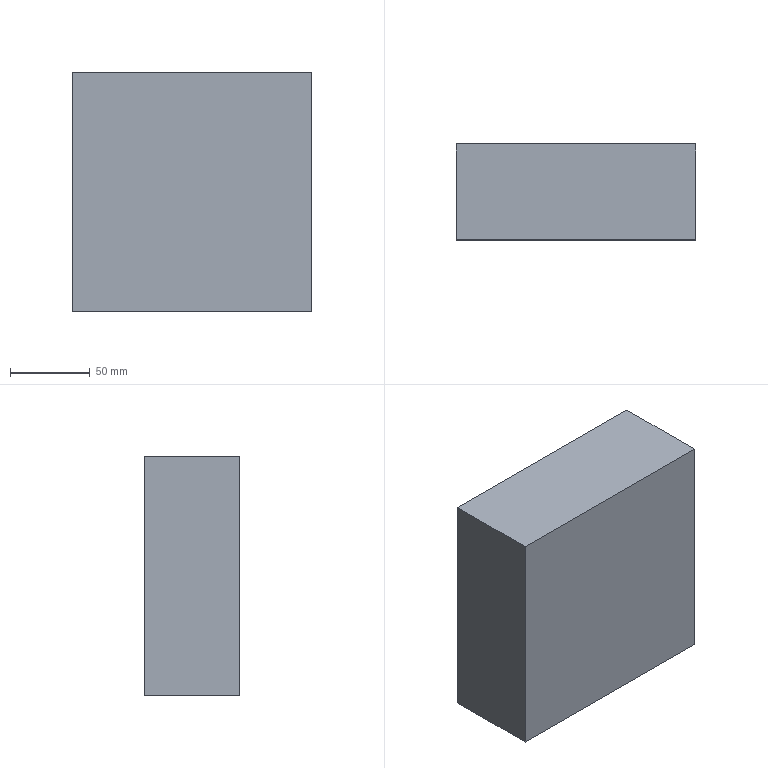Part | SolidWorks | features Extrusion 1 | 1 solid | 6 faces | box 150 x 60 x 150 mm | volume 1350000 mm3 | plane 6
STEP:
#1=CARTESIAN_POINT('',(75.,0.,75.));
#2=VERTEX_POINT('',#1);
#3=CARTESIAN_POINT('',(75.,0.,-75.));
#4=VERTEX_POINT('',#3);
#5=CARTESIAN_POINT('',(75.,0.,-75.));
#6=DIRECTION('',(0.,0.,-1.));
#7=VECTOR('',#6,1000.);
#8=LINE('',#5,#7);
#9=EDGE_CURVE('',#2,#4,#8,.T.);
#10=ORIENTED_EDGE('',*,*,#9,.T.);
#11=CARTESIAN_POINT('',(75.,60.,-75.));
#12=VERTEX_POINT('',#11);
#13=CARTESIAN_POINT('',(75.,60.,-75.));
#14=DIRECTION('',(0.,-1.,0.));
#15=VECTOR('',#14,1000.);
#16=LINE('',#13,#15);
#17=EDGE_CURVE('',#12,#4,#16,.T.);
#18=ORIENTED_EDGE('',*,*,#17,.F.);
#19=CARTESIAN_POINT('',(75.,60.,75.));
#20=VERTEX_POINT('',#19);
#21=CARTESIAN_POINT('',(75.,60.,-75.));
#22=DIRECTION('',(0.,0.,-1.));
#23=VECTOR('',#22,1000.);
#24=LINE('',#21,#23);
#25=EDGE_CURVE('',#20,#12,#24,.T.);
#26=ORIENTED_EDGE('',*,*,#25,.F.);
#27=CARTESIAN_POINT('',(75.,60.,75.));
#28=DIRECTION('',(0.,-1.,0.));
#29=VECTOR('',#28,1000.);
#30=LINE('',#27,#29);
#31=EDGE_CURVE('',#20,#2,#30,.T.);
#32=ORIENTED_EDGE('',*,*,#31,.T.);
#33=EDGE_LOOP('',(#10,#18,#26,#32));
#34=FACE_OUTER_BOUND('',#33,.T.);
#35=CARTESIAN_POINT('',(75.,60.,-75.));
#36=DIRECTION('',(-1.,0.,0.));
#37=DIRECTION('',(0.,0.,1.));
#38=AXIS2_PLACEMENT_3D('',#35,#36,#37);
#39=PLANE('',#38);
#40=ADVANCED_FACE('',(#34),#39,.F.);
#41=CARTESIAN_POINT('',(-75.,0.,-75.));
#42=VERTEX_POINT('',#41);
#43=CARTESIAN_POINT('',(-75.,0.,-75.));
#44=DIRECTION('',(-1.,0.,0.));
#45=VECTOR('',#44,1000.);
#46=LINE('',#43,#45);
#47=EDGE_CURVE('',#4,#42,#46,.T.);
#48=ORIENTED_EDGE('',*,*,#47,.T.);
#49=CARTESIAN_POINT('',(-75.,60.,-75.));
#50=VERTEX_POINT('',#49);
#51=CARTESIAN_POINT('',(-75.,60.,-75.));
#52=DIRECTION('',(0.,-1.,0.));
#53=VECTOR('',#52,1000.);
#54=LINE('',#51,#53);
#55=EDGE_CURVE('',#50,#42,#54,.T.);
#56=ORIENTED_EDGE('',*,*,#55,.F.);
#57=CARTESIAN_POINT('',(-75.,60.,-75.));
#58=DIRECTION('',(-1.,0.,0.));
#59=VECTOR('',#58,1000.);
#60=LINE('',#57,#59);
#61=EDGE_CURVE('',#12,#50,#60,.T.);
#62=ORIENTED_EDGE('',*,*,#61,.F.);
#63=ORIENTED_EDGE('',*,*,#17,.T.);
#64=EDGE_LOOP('',(#48,#56,#62,#63));
#65=FACE_OUTER_BOUND('',#64,.T.);
#66=CARTESIAN_POINT('',(-75.,60.,-75.));
#67=DIRECTION('',(0.,0.,1.));
#68=DIRECTION('',(1.,0.,0.));
#69=AXIS2_PLACEMENT_3D('',#66,#67,#68);
#70=PLANE('',#69);
#71=ADVANCED_FACE('',(#65),#70,.F.);
#72=CARTESIAN_POINT('',(-75.,0.,75.));
#73=VERTEX_POINT('',#72);
#74=CARTESIAN_POINT('',(-75.,0.,-75.));
#75=DIRECTION('',(0.,0.,1.));
#76=VECTOR('',#75,1000.);
#77=LINE('',#74,#76);
#78=EDGE_CURVE('',#42,#73,#77,.T.);
#79=ORIENTED_EDGE('',*,*,#78,.T.);
#80=CARTESIAN_POINT('',(-75.,60.,75.));
#81=VERTEX_POINT('',#80);
#82=CARTESIAN_POINT('',(-75.,60.,75.));
#83=DIRECTION('',(0.,-1.,0.));
#84=VECTOR('',#83,1000.);
#85=LINE('',#82,#84);
#86=EDGE_CURVE('',#81,#73,#85,.T.);
#87=ORIENTED_EDGE('',*,*,#86,.F.);
#88=CARTESIAN_POINT('',(-75.,60.,-75.));
#89=DIRECTION('',(0.,0.,1.));
#90=VECTOR('',#89,1000.);
#91=LINE('',#88,#90);
#92=EDGE_CURVE('',#50,#81,#91,.T.);
#93=ORIENTED_EDGE('',*,*,#92,.F.);
#94=ORIENTED_EDGE('',*,*,#55,.T.);
#95=EDGE_LOOP('',(#79,#87,#93,#94));
#96=FACE_OUTER_BOUND('',#95,.T.);
#97=CARTESIAN_POINT('',(-75.,60.,-75.));
#98=DIRECTION('',(1.,0.,0.));
#99=DIRECTION('',(0.,0.,-1.));
#100=AXIS2_PLACEMENT_3D('',#97,#98,#99);
#101=PLANE('',#100);
#102=ADVANCED_FACE('',(#96),#101,.F.);
#103=CARTESIAN_POINT('',(-75.,0.,75.));
#104=DIRECTION('',(1.,0.,0.));
#105=VECTOR('',#104,1000.);
#106=LINE('',#103,#105);
#107=EDGE_CURVE('',#73,#2,#106,.T.);
#108=ORIENTED_EDGE('',*,*,#107,.T.);
#109=ORIENTED_EDGE('',*,*,#31,.F.);
#110=CARTESIAN_POINT('',(-75.,60.,75.));
#111=DIRECTION('',(1.,0.,0.));
#112=VECTOR('',#111,1000.);
#113=LINE('',#110,#112);
#114=EDGE_CURVE('',#81,#20,#113,.T.);
#115=ORIENTED_EDGE('',*,*,#114,.F.);
#116=ORIENTED_EDGE('',*,*,#86,.T.);
#117=EDGE_LOOP('',(#108,#109,#115,#116));
#118=FACE_OUTER_BOUND('',#117,.T.);
#119=CARTESIAN_POINT('',(-75.,60.,75.));
#120=DIRECTION('',(0.,0.,-1.));
#121=DIRECTION('',(-1.,0.,0.));
#122=AXIS2_PLACEMENT_3D('',#119,#120,#121);
#123=PLANE('',#122);
#124=ADVANCED_FACE('',(#118),#123,.F.);
#125=ORIENTED_EDGE('',*,*,#25,.T.);
#126=ORIENTED_EDGE('',*,*,#61,.T.);
#127=ORIENTED_EDGE('',*,*,#92,.T.);
#128=ORIENTED_EDGE('',*,*,#114,.T.);
#129=EDGE_LOOP('',(#125,#126,#127,#128));
#130=FACE_OUTER_BOUND('',#129,.T.);
#131=CARTESIAN_POINT('',(0.,60.,0.));
#132=DIRECTION('',(0.,1.,0.));
#133=DIRECTION('',(0.,0.,1.));
#134=AXIS2_PLACEMENT_3D('',#131,#132,#133);
#135=PLANE('',#134);
#136=ADVANCED_FACE('',(#130),#135,.T.);
#137=ORIENTED_EDGE('',*,*,#9,.F.);
#138=ORIENTED_EDGE('',*,*,#107,.F.);
#139=ORIENTED_EDGE('',*,*,#78,.F.);
#140=ORIENTED_EDGE('',*,*,#47,.F.);
#141=EDGE_LOOP('',(#137,#138,#139,#140));
#142=FACE_OUTER_BOUND('',#141,.T.);
#143=CARTESIAN_POINT('',(0.,0.,0.));
#144=DIRECTION('',(0.,1.,0.));
#145=DIRECTION('',(0.,0.,1.));
#146=AXIS2_PLACEMENT_3D('',#143,#144,#145);
#147=PLANE('',#146);
#148=ADVANCED_FACE('',(#142),#147,.F.);
#149=CLOSED_SHELL('',(#40,#71,#102,#124,#136,#148));
#150=MANIFOLD_SOLID_BREP('',#149);
#151=CARTESIAN_POINT('',(0.,0.,0.));
#152=DIRECTION('',(0.,0.,1.));
#153=DIRECTION('',(1.,0.,0.));
#154=AXIS2_PLACEMENT_3D('',#151,#152,#153);
#155=(LENGTH_UNIT()NAMED_UNIT(*)SI_UNIT(.MILLI.,.METRE.));
#156=UNCERTAINTY_MEASURE_WITH_UNIT(LENGTH_MEASURE(0.00001),#155,'','');
#157=(NAMED_UNIT(*)PLANE_ANGLE_UNIT()SI_UNIT($,.RADIAN.));
#158=(NAMED_UNIT(*)SI_UNIT($,.STERADIAN.)SOLID_ANGLE_UNIT());
#159=(GEOMETRIC_REPRESENTATION_CONTEXT(3)GLOBAL_UNCERTAINTY_ASSIGNED_CONTEXT((#156))GLOBAL_UNIT_ASSIGNED_CONTEXT((#155,#157,#158))REPRESENTATION_CONTEXT('',''));
#160=ADVANCED_BREP_SHAPE_REPRESENTATION('',(#150,#154),#159);